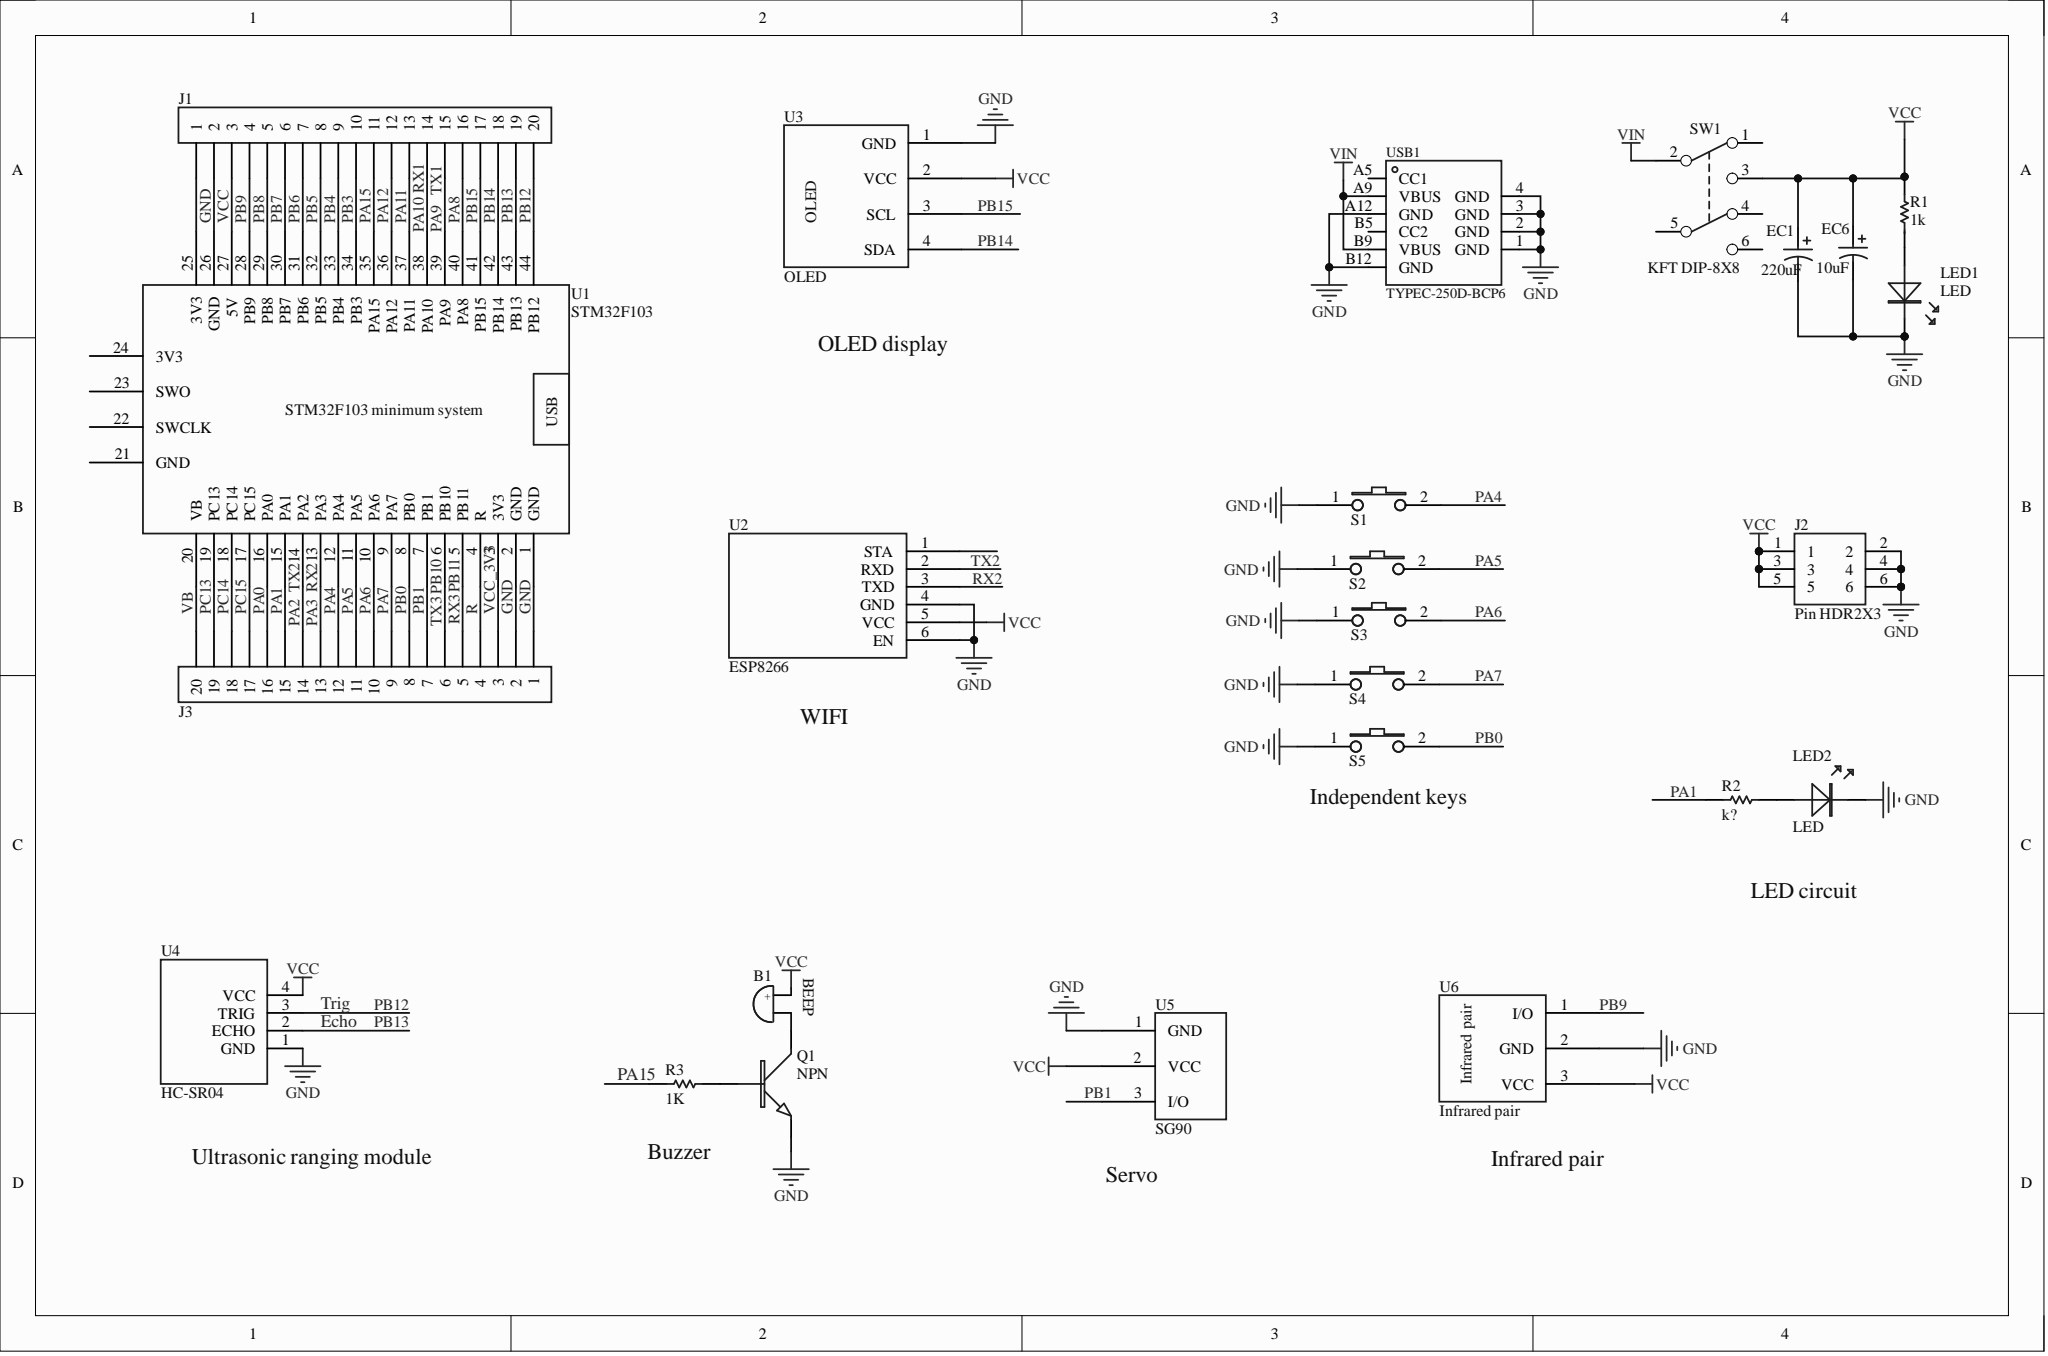Circuit board | Altium Designer | 25 parts | 43 nets
Bill of materials:
Comment,Description,Designator,Footprint,LibRef,Quantity
"BEEP","Buzzer","B1","BEEP 7.6X12X7.5","BEEP","1"
"220uF","Polarized capacitor","EC1","DIP-EC2.5X5X11","220uF","1"
"10uF","Polarized capacitor","EC6","DIP-EC2.5X5X11","10uF","1"
"","","J1, J3","Pin HDR1X20/2.54mm-S","J1, J3","2"
"Pin HDR2X3","","J2","Pin HDR2X3/2.54mm-S","Pin HDR2X3","1"
"LED","","LED1, LED2","LED5-BLUE","LED","2"
"NPN","NPN transistor","Q1","TO-92A","NPN","1"
"1k","","R1, R3","AXIAL0.3","1k","2"
"k?","","R2","AXIAL0.3","k?","1"
"BUTTOM","Button","S1, S2, S3, S4, S5","DIP-6X6X5","BUTTOM","5"
"KFT DIP-8X8","","SW1","KFT DIP-8X8","KFT DIP-8X8","1"
"STM32F103","STM32F103","U1","STM32FF103","STM32F103","1"
"ESP8266","","U2","ECB02","ESP8266","1"
"OLED","OLED","U3","OLED","OLED","1"
"HC-SR04","Ultrasonic module","U4","超声波MODE","HC-SR04","1"
"SG90","SG90","U5","SG90","SG90","1"
"Infrared pair","Infrared pair","U6","红外对管","红外对管","1"
"TYPEC-250D-BCP6","","USB1","TYP-C-6","TYPEC-250D-BCP6","1"
Netlist (Protel format):
[
B1
BEEP 7.6X12X7.5
BEEP



]
[
EC1
DIP-EC2.5X5X11
220uF



]
[
EC6
DIP-EC2.5X5X11
10uF



]
[
J1
Pin HDR1X20/2.54mm-S




]
[
J2
Pin HDR2X3/2.54mm-S
Pin HDR2X3



]
[
J3
Pin HDR1X20/2.54mm-S




]
[
LED1
LED5-BLUE
LED



]
[
LED2
LED5-BLUE
LED



]
[
Q1
TO-92A
NPN



]
[
R1
AXIAL0.3
1k



]
[
R2
AXIAL0.3
k?



]
[
R3
AXIAL0.3
1K



]
[
S1
DIP-6X6X5
BUTTOM



]
[
S2
DIP-6X6X5
BUTTOM



]
[
S3
DIP-6X6X5
BUTTOM



]
[
S4
DIP-6X6X5
BUTTOM



]
[
S5
DIP-6X6X5
BUTTOM



]
[
SW1
KFT DIP-8X8
KFT DIP-8X8



]
[
U1
STM32FF103
STM32F103



]
[
U2
ECB02
ESP8266



]
[
U3
OLED
OLED



]
[
U4
超声波MODE
HC-SR04



]
[
U5
SG90
SG90



]
[
U6
红外对管
Infrared pair



]
[
USB1
TYP-C-6
TYPEC-250D-BCP6



]
(
VIN
SW1-2
USB1-A9
USB1-B9
)
(
VCC_3V3
J3-3
U1-3
)
(
VCC
B1-1
EC1-1
EC6-1
J1-3
J2-1
J2-3
J2-5
R1-2
SW1-3
U1-27
U2-5
U3-2
U4-4
U5-2
U6-3
)
(
VB
J3-20
U1-20
)
(
R
J3-4
U1-4
)
(
PC15
J3-17
U1-17
)
(
PC14
J3-18
U1-18
)
(
PC13
J3-19
U1-19
)
(
PB15
J1-17
U1-41
U3-3
)
(
PB14
J1-18
U1-42
U3-4
)
(
PB12
J1-20
U1-44
U4-3
)
(
PB11
J3-5
U1-5
)
(
PB10
J3-6
U1-6
)
(
PB9
J1-4
U1-28
U6-1
)
(
PB8
J1-5
U1-29
)
(
PB7
J1-6
U1-30
)
(
PB6
J1-7
U1-31
)
(
PB5
J1-8
U1-32
)
(
PB4
J1-9
U1-33
)
(
PB3
J1-10
U1-34
)
(
PB1
J3-7
U1-7
U5-3
)
(
PB0
J3-8
S5-2
U1-8
)
(
PA15
J1-11
R3-1
U1-35
)
(
PA12
J1-12
U1-36
)
(
PA11
J1-13
U1-37
)
(
PA10
J1-14
U1-38
)
(
PA9
J1-15
U1-39
)
(
PA8
J1-16
U1-40
)
(
PA7
J3-9
S4-2
U1-9
)
(
PA6
J3-10
S3-2
U1-10
)
(
PA5
J3-11
S2-2
U1-11
)
(
PA4
J3-12
S1-2
U1-12
)
(
PA3
J3-13
U1-13
U2-3
)
(
PA2
J3-14
U1-14
U2-2
)
(
PA1
J3-15
R2-1
U1-15
)
(
PA0
J3-16
U1-16
)
(
NetQ1_B
Q1-B
R3-2
)
(
NetLED2_A
LED2-A
R2-2
)
(
NetLED1_A
LED1-A
R1-1
)
(
NetJ1_1
J1-1
U1-25
)
(
NetB1_2
B1-2
Q1-C
)
(
GND
EC1-2
EC6-2
J1-2
J2-2
J2-4
J2-6
J3-1
J3-2
LED1-K
LED2-K
Q1-E
S1-1
S2-1
S3-1
S4-1
S5-1
U1-1
U1-2
U1-26
U2-4
U2-6
U3-1
U4-1
U5-1
U6-2
USB1-1
USB1-2
USB1-3
USB1-4
USB1-A12
USB1-B12
)
(
Echo
J1-19
U1-43
U4-2
)